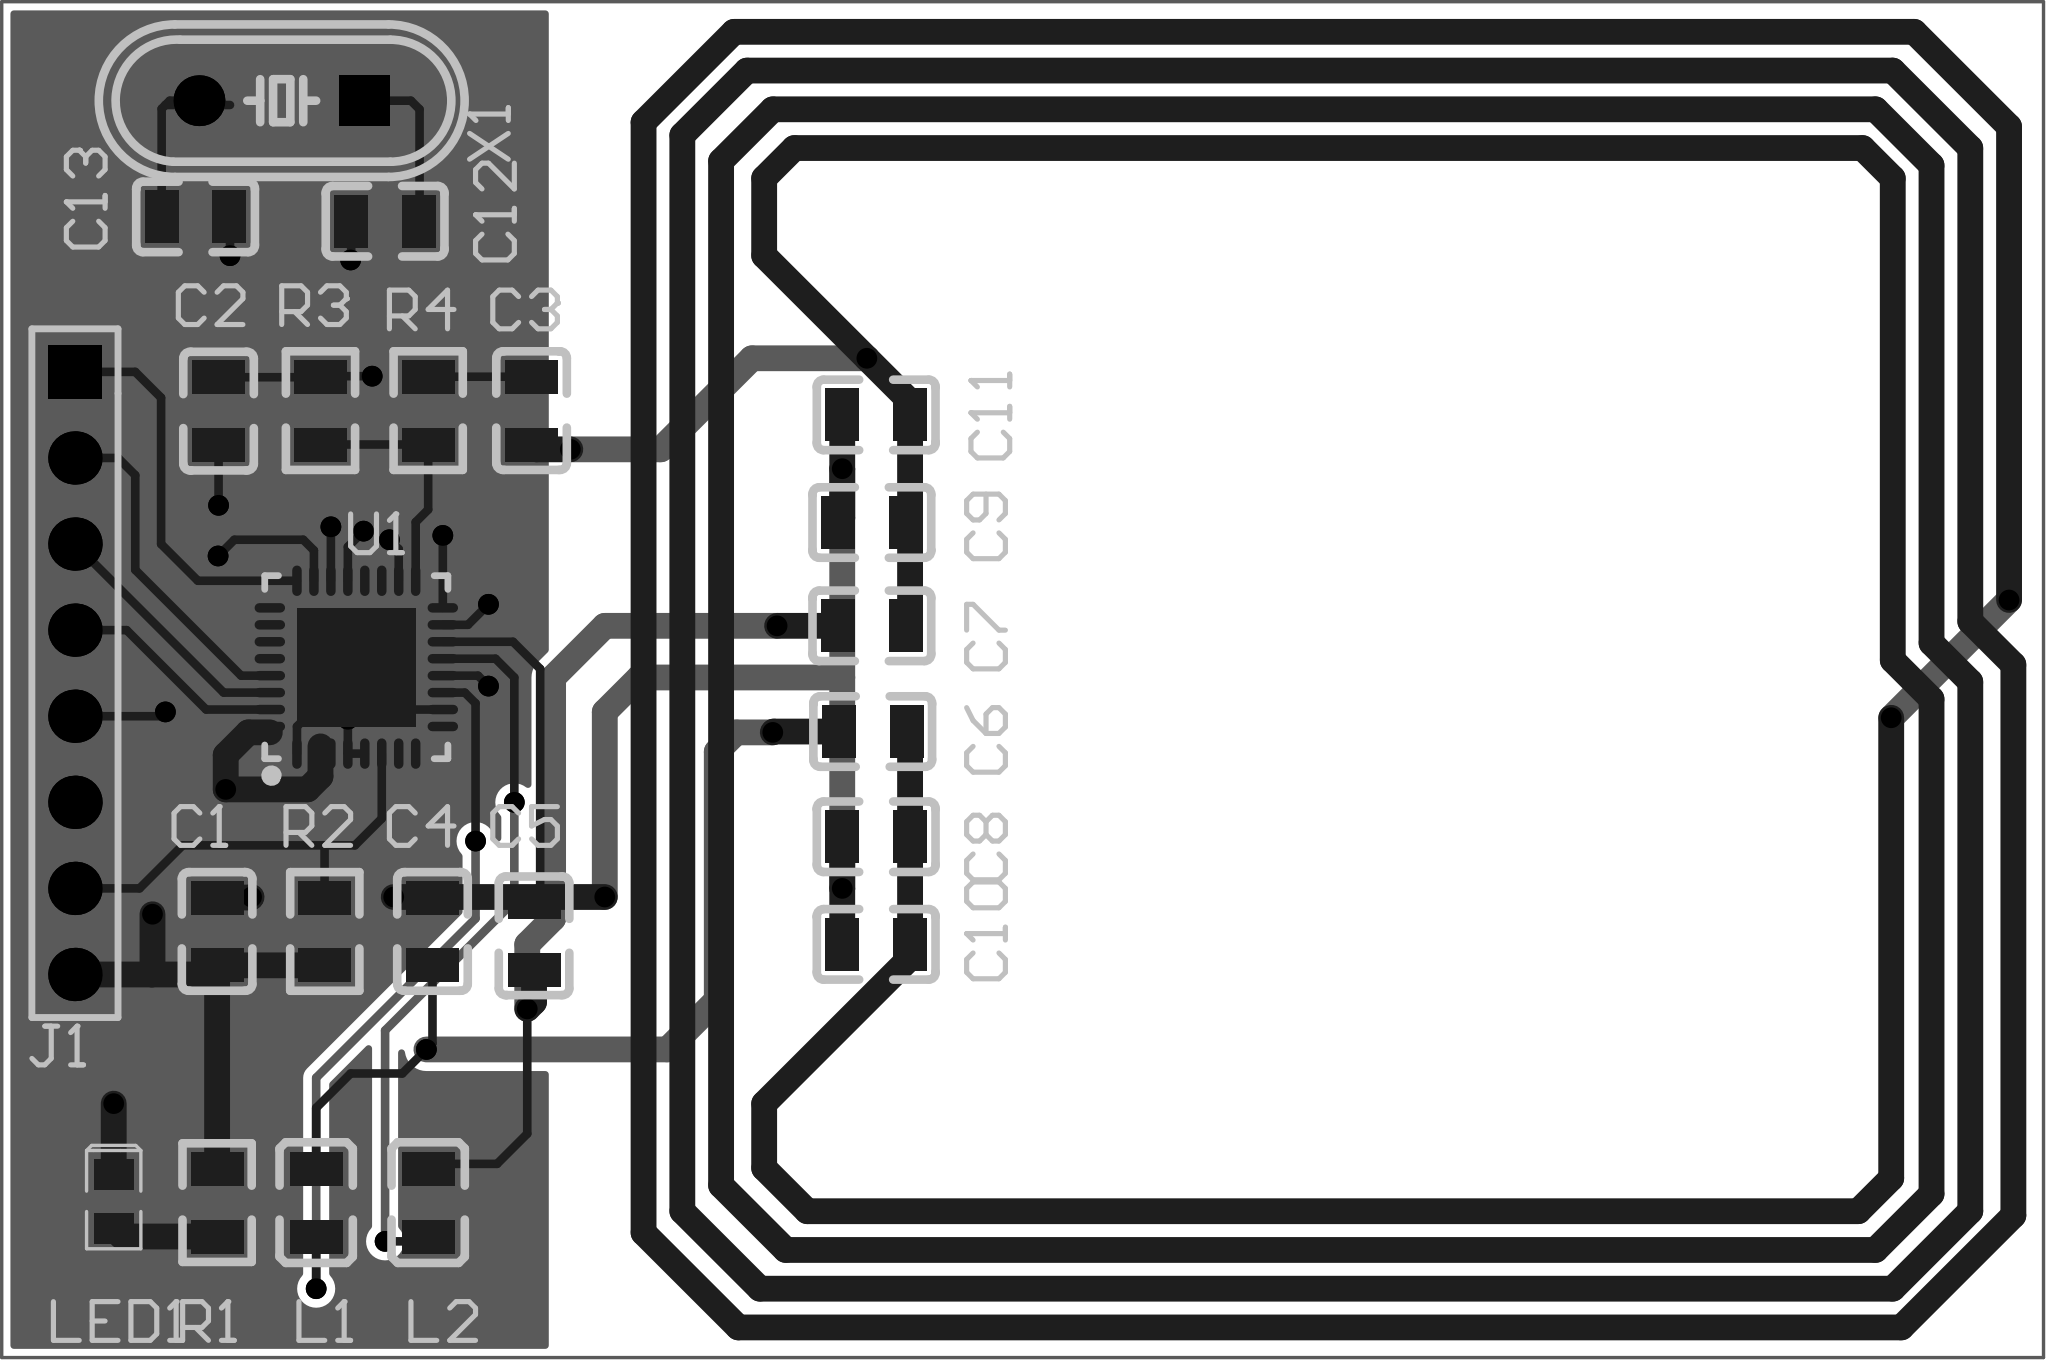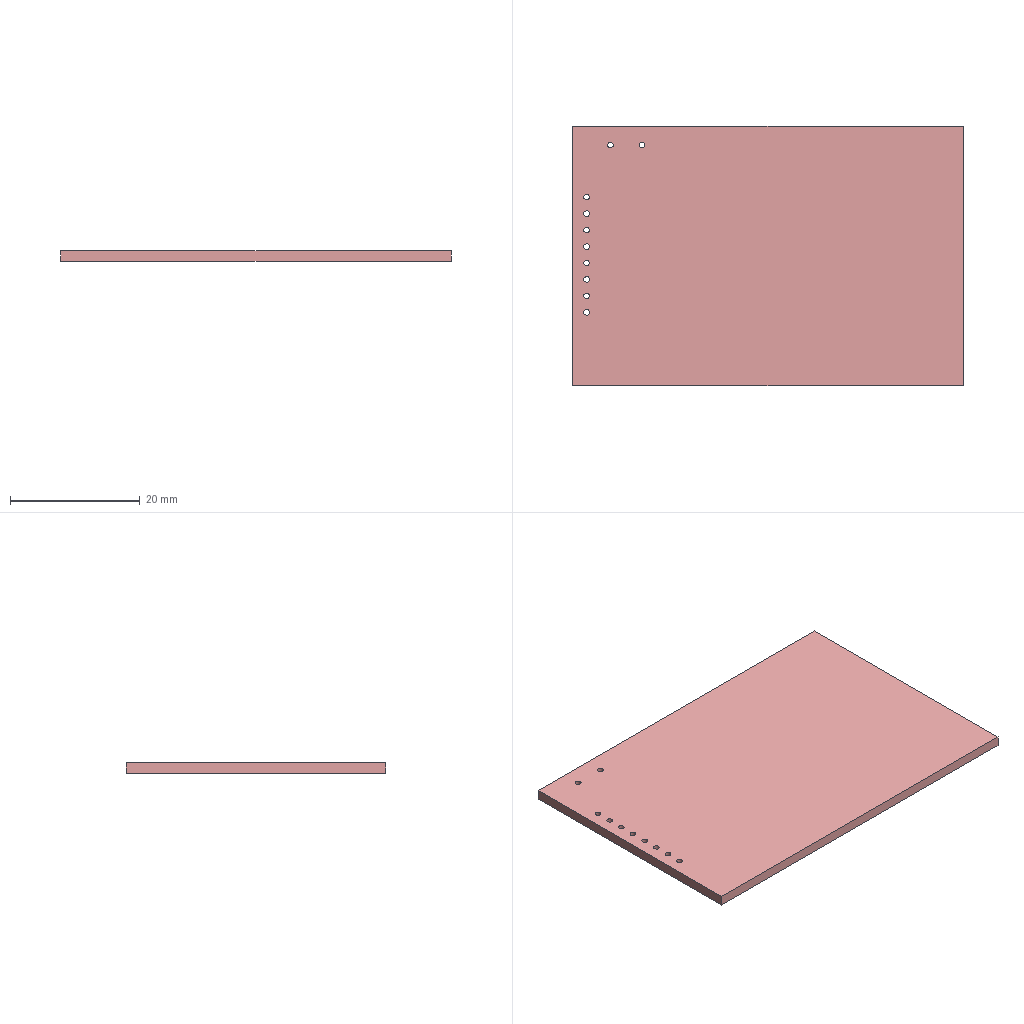Circuit board layout | Altium Designer | box 60.2 x 40 x 1.6 mm
Layer stack:
# Altium Designer layer stack of  (unit mm; dielectric type: 0 none, 1 core, 2 prepreg, 3 surface material)
index,name,kind,layer,copper_thickness_mm,dielectric_type,dielectric_thickness_mm,dielectric_material,dielectric_constant
0,Top Paste Mask Layer,other,,,,,,
1,Top Silkscreen Layer,other,,,,,,
2,Top Solder Mask Layer,dielectric,,,3,0.01,,3.3
3,Top Layer,copper,Top Layer,0.035,,,,
4,Dielectric1,dielectric,,,3,1.51,FR4,4.5
5,Bottom Layer,copper,Bottom Layer,0.035,,,,
6,Bottom Solder Mask Layer,dielectric,,,3,0.01,,3.3
7,Bottom Silkscreen Layer,other,,,,,,
8,Bottom Paste Mask Layer,other,,,,,,
# drill layer pairs: low layer,high layer
drill_pair,Top Layer,Bottom Layer
Part placement:
Designator,Comment,Layer,Footprint,Center-X(mm),Center-Y(mm),Rotation
LED1,LED-0805_G,TopLayer,LED-0805_G,81.026,83.731,270
C13,15P,TopLayer,C0805,83.439,112.776,0
C1,0.1u,TopLayer,C0805,84.074,91.694,270
R1,1k,TopLayer,R0805,84.074,83.693,270
C2,0.1u,TopLayer,C0805,84.117,107.046,90
U1,MF522 COPY,TopLayer,LC-QFN-32_5X5X05P,88.179,99.491,0
L1,2.2uH,TopLayer,L0805,86.995,83.693,90
R3,820,TopLayer,R0805,87.122,107.061,270
R2,10K,TopLayer,R0805,87.249,91.694,90
C12,15P,TopLayer,C0805,89.027,112.649,180
L2,2.2uH,TopLayer,L0805,90.297,83.693,90
R4,5.1k,TopLayer,R0805,90.297,107.061,90
C4,47P,TopLayer,C0805,90.424,91.694,270
C3,0.1u,TopLayer,C0805,93.345,107.061,270
C5,47P,TopLayer,C0805,93.418,91.565,90
C7,15P,TopLayer,C0805,103.378,100.711,0
C9,10pf,TopLayer,C0805,103.378,103.759,180
C6,15P,TopLayer,C0805,103.403,97.592,0
C10,180P,TopLayer,C0805,103.505,91.313,0
C8,10pf,TopLayer,C0805,103.505,94.488,0
C11,180P,TopLayer,C0805,103.505,106.934,180
J1,HDR-M-2.54_1x8,TopLayer,HDR-M-2.54_1X8,79.883,99.314,270
X1,27.12MHz,TopLayer,HC-49US_L11.5-W4.5-P4.88,85.979,116.205,180
Pad and via stacks:
# Altium Designer via and pad stacks of  (unit mm). Each distinct definition once, with the count of objects using it.
# via: kind,start_layer,end_layer,hole_mm,diameter_mm,mode(0 simple;1 top-mid-bottom;2 full stack),diameter_per_layer,count,example_net
# pad: kind,layer,hole_mm,hole_type(0 round;1 square;2 slot),plating,top_size,top_shape(1 round;2 rect;3 octagon;9 rounded rect),mid_size,bottom_size,mode,footprint,size_per_layer,count,example
pad,Top Layer,0,0,plated,0.9x1.15,2,0.9x1.15,0.9x1.15,0,LED-0805_G,,2,LED1.1
pad,Top Layer,0,0,plated,1x1.55,2,1x1.55,1x1.55,0,C0805,,26,C13.1
pad,Top Layer,0,0,plated,1x1.55,2,1x1.55,1x1.55,0,R0805,,8,R1.2
pad,Top Layer,0,0,plated,3.5x3.5,2,3.5x3.5,3.5x3.5,0,LC-QFN-32_5X5X05P,,1,U1.0
pad,Top Layer,0,0,plated,0.2799x0.8999,1,0.2799x0.8999,0.2799x0.8999,0,LC-QFN-32_5X5X05P,,32,U1.1
pad,Top Layer,0,0,plated,1x1.55,2,1x1.55,1x1.55,0,L0805,,4,L1.2
pad,Multi-Layer,0.889,0,plated,1.575x1.575,2,1.575x1.575,1.575x1.575,0,HDR-M-2.54_1X8,,1,J1.1
pad,Multi-Layer,0.889,0,plated,1.575x1.575,1,1.575x1.575,1.575x1.575,0,HDR-M-2.54_1X8,,7,J1.2
pad,Multi-Layer,0.9,0,plated,1.5x1.5,2,1.5x1.5,1.5x1.5,0,HC-49US_L11.5-W4.5-P4.88,,1,X1.1
pad,Multi-Layer,0.9,0,plated,1.5x1.5,1,1.5x1.5,1.5x1.5,0,HC-49US_L11.5-W4.5-P4.88,,1,X1.2
via,Top Layer,Bottom Layer,0.3048,0.61,0,,39,GND
Copper pours:
name,layer,net,type(0 solid;1 hatched;2 none)
Bottom Layer-GND,Bottom Layer,GND,0
Design rules, without the lines most boards share:
# Altium Designer design rules of  (exported by Altium Designer, unit mm)
# columns: name | kind | enabled | priority | scope1 | scope2 | descriptor | typed fields (field=value)
creepage | 65 | enabled | 1 | All | All | Creepage Distance Constraint =(0mil) (All),(All) |